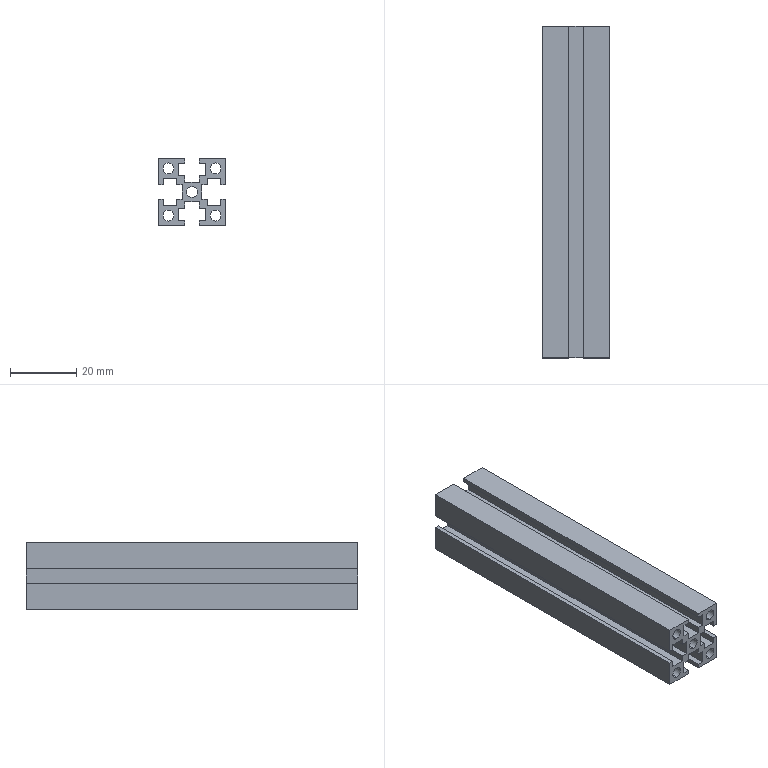Part | STEP file | 20 aluminium profile longitudinal 1 | 1 solid | 64 faces | box 20 x 100 x 20 mm | volume 17778 mm3 | plane 54 | cylinder 10 | commonest cylinder face diameters 3.3 x10